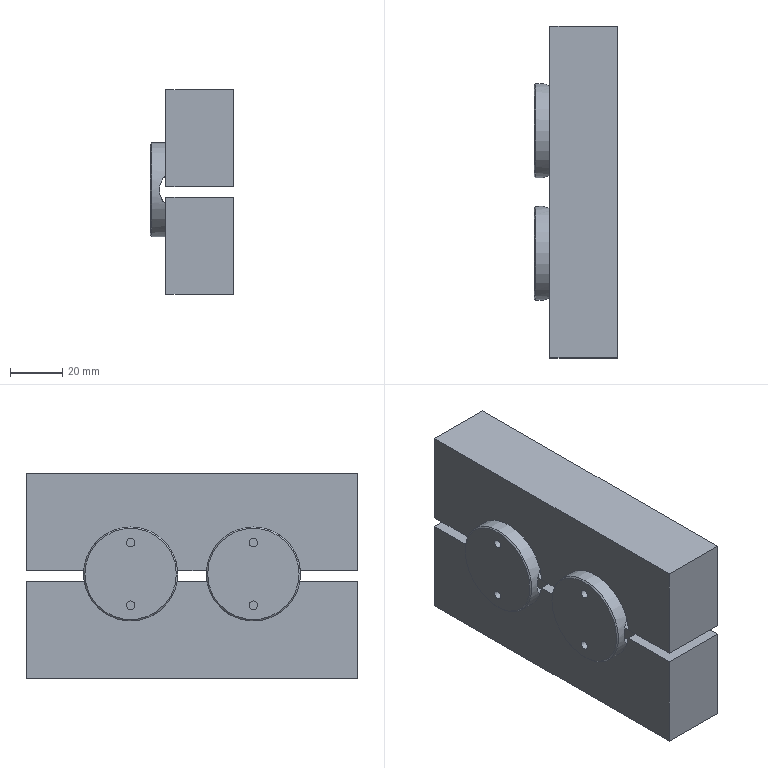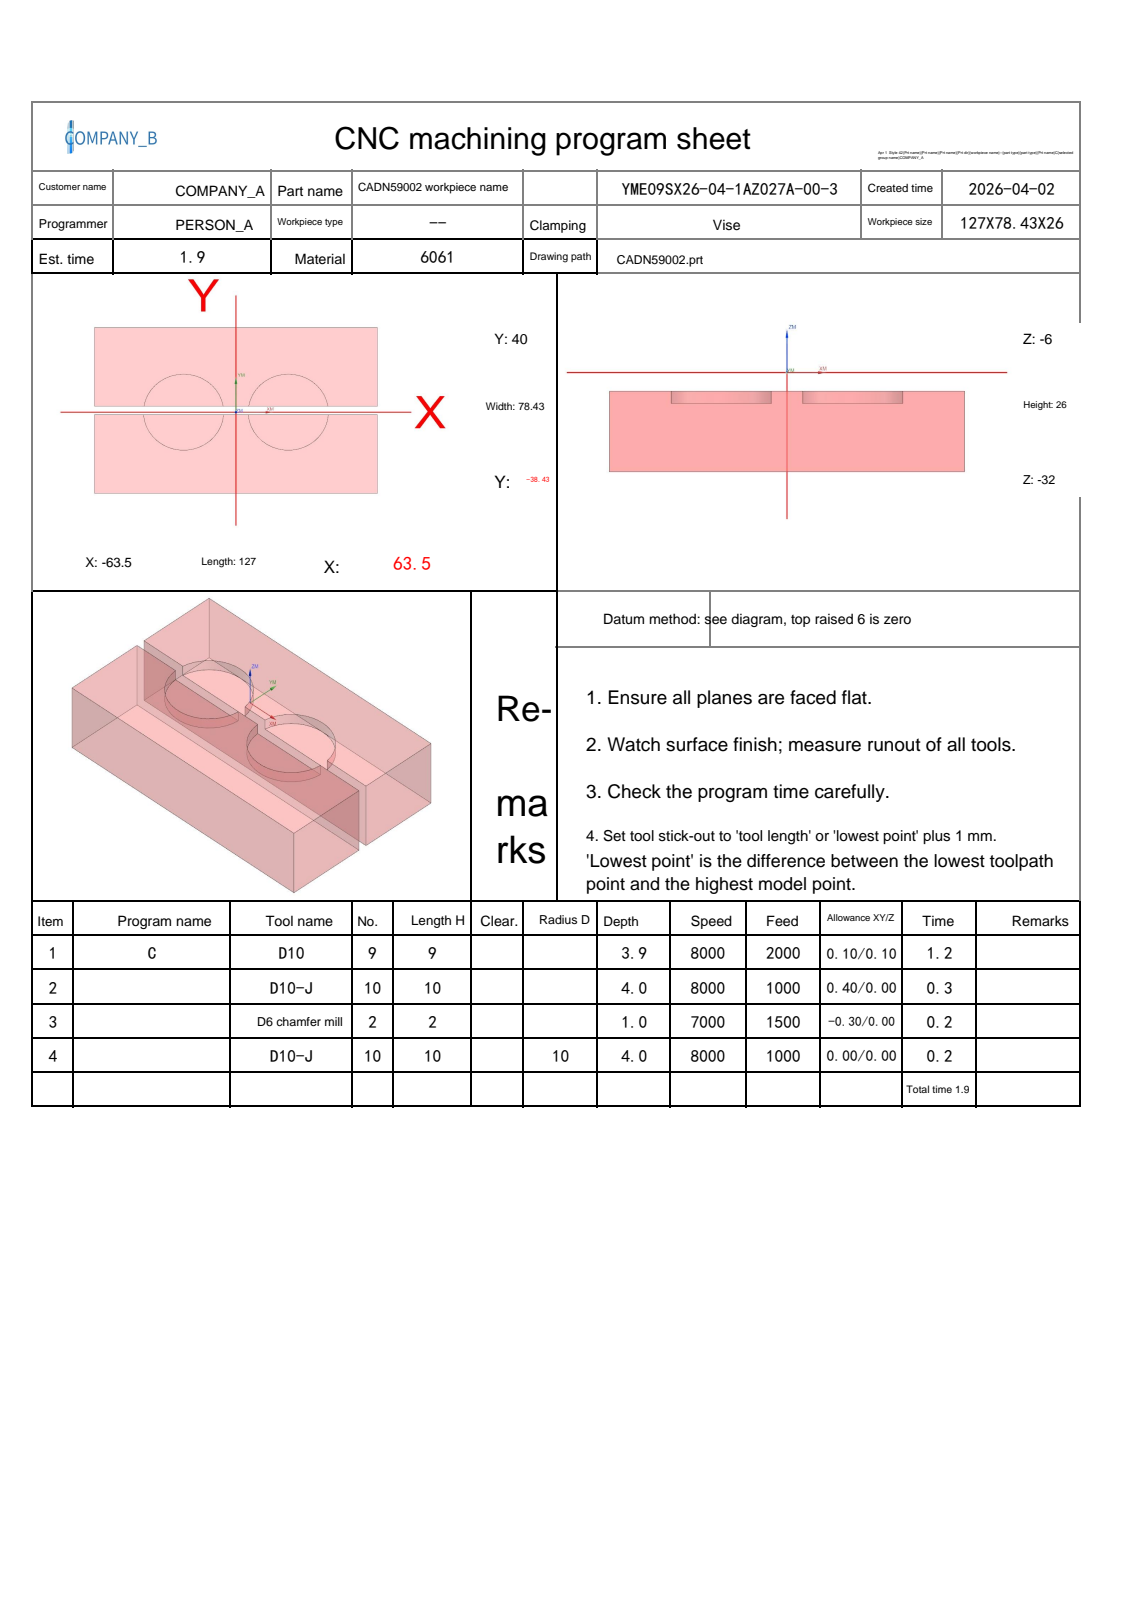NC program | NX | posted by the shop | part box 32 x 127 x 78.432 mm
Whole program:
%
O0001
(Machine time: 2.76 MIN)
(===Total Tool:3===)
(T9=D10     D=10.  R=0.   D-  H09 Z=-9.9  )
(T10=D10-J  D=10.  R=0.   D-  H10 Z=-10.  )
(T2=D6 chamfer mill   D=6.   R=0.   D-  H02 Z=-7.   )
G80 G90 G17 G49 G40
G91 G28 Z0
M01
N1 T09 M06
(D10  D=10. R=0. H=09 ce=0.10 di=0.10)
G00 G90 G54 X20.594 Y7.536 M03 S8000
G43 H09 Z4.1
M08
Z-4.5
G03 X20.594 Y7.536 Z-5.982 I2.906 J-3.436 F2000.
X23.5 Y-.4 Z-6.557 I2.906 J-3.436
G01 X23.527 Y-.399
G03 X23.9 Y0.0 I-.027 J.399
X23.5 Y.4 I-.4 J0.0
X23.1 Y0.0 I0.0 J-.4
G01 Y-.006
X23.11 Y-.041
X25.447 Y-4.037
G03 X26.224 Y-4.482 I.777 J.454
X26.768 Y-4.299 I0.0 J.9
X28.888 Y-.364 I-3.268 J4.299
G01 X28.921 Y.128
X28.923 Y.194
X28.911 Y.347
X28.835 Y.835
G03 X23.5 Y5.4 I-5.335 J-.835
X18.165 Y.834 I0.0 J-5.4
G01 X18.089 Y.347
X18.077 Y.194
X18.079 Y.128
X18.112 Y-.365
G03 X20.87 Y-4.716 I5.388 J.365
G02 X21.231 Y-5.059 I-.487 J-.873
G01 X25.608 Y-12.058
G03 X26.456 Y-12.527 I.848 J.531
X26.704 Y-12.496 I0.0 J1.
X36.371 Y-.871 I-3.204 J12.496
G01 X36.468 Y.569
X36.245 Y1.995
G03 X23.5 Y12.9 I-12.745 J-1.995
X10.755 Y1.995 I0.0 J-12.9
G01 X10.532 Y.569
X10.629 Y-.871
G03 X23.5 Y-12.9 I12.871 J.871
X28.376 Y-11.943 I0.0 J12.9
X28.835 Y-11.745 I-4.876 J11.943
G01 X27.594 Y-9.014
Z-5.057
G00 X20.594 Y7.536
G03 X20.594 Y7.536 Z-6.539 I2.906 J-3.436
X23.5 Y-.4 Z-7.114 I2.906 J-3.436
G01 X23.527 Y-.399
G03 X23.9 Y0.0 I-.027 J.399
X23.5 Y.4 I-.4 J0.0
X23.1 Y0.0 I0.0 J-.4
G01 Y-.006
X23.11 Y-.041
X25.447 Y-4.037
G03 X26.224 Y-4.482 I.777 J.454
X26.768 Y-4.299 I0.0 J.9
X28.888 Y-.364 I-3.268 J4.299
G01 X28.921 Y.128
X28.923 Y.194
X28.911 Y.347
X28.835 Y.835
G03 X23.5 Y5.4 I-5.335 J-.835
X18.165 Y.834 I0.0 J-5.4
G01 X18.089 Y.347
X18.077 Y.194
X18.079 Y.128
X18.112 Y-.365
G03 X20.87 Y-4.716 I5.388 J.365
G02 X21.231 Y-5.059 I-.487 J-.873
G01 X25.608 Y-12.058
G03 X26.456 Y-12.527 I.848 J.531
X26.704 Y-12.496 I0.0 J1.
X36.371 Y-.871 I-3.204 J12.496
G01 X36.468 Y.569
X36.245 Y1.995
G03 X23.5 Y12.9 I-12.745 J-1.995
X10.755 Y1.995 I0.0 J-12.9
G01 X10.532 Y.569
X10.629 Y-.871
G03 X23.5 Y-12.9 I12.871 J.871
X28.376 Y-11.943 I0.0 J12.9
X28.835 Y-11.745 I-4.876 J11.943
G01 X27.594 Y-9.014
Z-5.614
G00 X20.594 Y7.536
G03 X20.594 Y7.536 Z-7.096 I2.906 J-3.436
X23.5 Y-.4 Z-7.671 I2.906 J-3.436
G01 X23.527 Y-.399
G03 X23.9 Y0.0 I-.027 J.399
X23.5 Y.4 I-.4 J0.0
X23.1 Y0.0 I0.0 J-.4
G01 Y-.006
X23.11 Y-.041
X25.447 Y-4.037
G03 X26.224 Y-4.482 I.777 J.454
X26.768 Y-4.299 I0.0 J.9
X28.888 Y-.364 I-3.268 J4.299
G01 X28.921 Y.128
X28.923 Y.194
X28.911 Y.347
X28.835 Y.835
G03 X23.5 Y5.4 I-5.335 J-.835
X18.165 Y.834 I0.0 J-5.4
G01 X18.089 Y.347
X18.077 Y.194
X18.079 Y.128
X18.112 Y-.365
G03 X20.87 Y-4.716 I5.388 J.365
G02 X21.231 Y-5.059 I-.487 J-.873
G01 X25.608 Y-12.058
G03 X26.456 Y-12.527 I.848 J.531
X26.704 Y-12.496 I0.0 J1.
X36.371 Y-.871 I-3.204 J12.496
G01 X36.468 Y.569
X36.245 Y1.995
G03 X23.5 Y12.9 I-12.745 J-1.995
X10.755 Y1.995 I0.0 J-12.9
G01 X10.532 Y.569
X10.629 Y-.871
G03 X23.5 Y-12.9 I12.871 J.871
X28.376 Y-11.943 I0.0 J12.9
X28.835 Y-11.745 I-4.876 J11.943
G01 X27.594 Y-9.014
Z-6.171
G00 X20.594 Y7.536
G03 X20.594 Y7.536 Z-7.653 I2.906 J-3.436
X23.5 Y-.4 Z-8.229 I2.906 J-3.436
G01 X23.527 Y-.399
G03 X23.9 Y0.0 I-.027 J.399
X23.5 Y.4 I-.4 J0.0
X23.1 Y0.0 I0.0 J-.4
G01 Y-.006
X23.11 Y-.041
X25.447 Y-4.037
G03 X26.224 Y-4.482 I.777 J.454
X26.768 Y-4.299 I0.0 J.9
X28.888 Y-.364 I-3.268 J4.299
G01 X28.921 Y.128
X28.923 Y.194
X28.911 Y.347
X28.835 Y.835
G03 X23.5 Y5.4 I-5.335 J-.835
X18.165 Y.834 I0.0 J-5.4
G01 X18.089 Y.347
X18.077 Y.194
X18.079 Y.128
X18.112 Y-.365
G03 X20.87 Y-4.716 I5.388 J.365
G02 X21.231 Y-5.059 I-.487 J-.873
G01 X25.608 Y-12.058
G03 X26.456 Y-12.527 I.848 J.531
X26.704 Y-12.496 I0.0 J1.
X36.371 Y-.871 I-3.204 J12.496
G01 X36.468 Y.569
X36.245 Y1.995
G03 X23.5 Y12.9 I-12.745 J-1.995
X10.755 Y1.995 I0.0 J-12.9
G01 X10.532 Y.569
X10.629 Y-.871
G03 X23.5 Y-12.9 I12.871 J.871
X28.376 Y-11.943 I0.0 J12.9
X28.835 Y-11.745 I-4.876 J11.943
G01 X27.594 Y-9.014
Z-6.729
G00 X20.594 Y7.536
G03 X20.594 Y7.536 Z-8.21 I2.906 J-3.436
X23.5 Y-.4 Z-8.786 I2.906 J-3.436
G01 X23.527 Y-.399
G03 X23.9 Y0.0 I-.027 J.399
X23.5 Y.4 I-.4 J0.0
X23.1 Y0.0 I0.0 J-.4
G01 Y-.006
X23.11 Y-.041
X25.447 Y-4.037
G03 X26.224 Y-4.482 I.777 J.454
X26.768 Y-4.299 I0.0 J.9
X28.888 Y-.364 I-3.268 J4.299
G01 X28.921 Y.128
X28.923 Y.194
X28.911 Y.347
X28.835 Y.835
G03 X23.5 Y5.4 I-5.335 J-.835
X18.165 Y.834 I0.0 J-5.4
G01 X18.089 Y.347
X18.077 Y.194
X18.079 Y.128
X18.112 Y-.365
G03 X20.87 Y-4.716 I5.388 J.365
G02 X21.231 Y-5.059 I-.487 J-.873
G01 X25.608 Y-12.058
G03 X26.456 Y-12.527 I.848 J.531
X26.704 Y-12.496 I0.0 J1.
X36.371 Y-.871 I-3.204 J12.496
G01 X36.468 Y.569
X36.245 Y1.995
G03 X23.5 Y12.9 I-12.745 J-1.995
X10.755 Y1.995 I0.0 J-12.9
G01 X10.532 Y.569
X10.629 Y-.871
G03 X23.5 Y-12.9 I12.871 J.871
X28.376 Y-11.943 I0.0 J12.9
X28.835 Y-11.745 I-4.876 J11.943
G01 X27.594 Y-9.014
Z-7.286
G00 X20.594 Y7.536
G03 X20.594 Y7.536 Z-8.768 I2.906 J-3.436
X23.5 Y-.4 Z-9.343 I2.906 J-3.436
G01 X23.527 Y-.399
G03 X23.9 Y0.0 I-.027 J.399
X23.5 Y.4 I-.4 J0.0
X23.1 Y0.0 I0.0 J-.4
G01 Y-.006
X23.11 Y-.041
X25.447 Y-4.037
G03 X26.224 Y-4.482 I.777 J.454
X26.768 Y-4.299 I0.0 J.9
X28.888 Y-.364 I-3.268 J4.299
G01 X28.921 Y.128
X28.923 Y.194
X28.911 Y.347
X28.835 Y.835
G03 X23.5 Y5.4 I-5.335 J-.835
X18.165 Y.834 I0.0 J-5.4
G01 X18.089 Y.347
X18.077 Y.194
X18.079 Y.128
X18.112 Y-.365
G03 X20.87 Y-4.716 I5.388 J.365
G02 X21.231 Y-5.059 I-.487 J-.873
G01 X25.608 Y-12.058
G03 X26.456 Y-12.527 I.848 J.531
X26.704 Y-12.496 I0.0 J1.
X36.371 Y-.871 I-3.204 J12.496
G01 X36.468 Y.569
X36.245 Y1.995
G03 X23.5 Y12.9 I-12.745 J-1.995
X10.755 Y1.995 I0.0 J-12.9
G01 X10.532 Y.569
X10.629 Y-.871
G03 X23.5 Y-12.9 I12.871 J.871
X28.376 Y-11.943 I0.0 J12.9
X28.835 Y-11.745 I-4.876 J11.943
G01 X27.594 Y-9.014
Z-7.843
G00 X20.594 Y7.536
G03 X20.594 Y7.536 Z-9.325 I2.906 J-3.436
X23.5 Y-.4 Z-9.9 I2.906 J-3.436
G01 X23.527 Y-.399
G03 X23.9 Y0.0 I-.027 J.399
X23.5 Y.4 I-.4 J0.0
X23.1 Y0.0 I0.0 J-.4
G01 Y-.006
X23.11 Y-.041
X25.447 Y-4.037
G03 X26.224 Y-4.482 I.777 J.454
X26.768 Y-4.299 I0.0 J.9
X28.888 Y-.364 I-3.268 J4.299
G01 X28.921 Y.128
X28.923 Y.194
X28.911 Y.347
X28.835 Y.835
G03 X23.5 Y5.4 I-5.335 J-.835
X18.165 Y.834 I0.0 J-5.4
G01 X18.089 Y.347
X18.077 Y.194
X18.079 Y.128
X18.112 Y-.365
G03 X20.87 Y-4.716 I5.388 J.365
G02 X21.231 Y-5.059 I-.487 J-.873
G01 X25.608 Y-12.058
G03 X26.456 Y-12.527 I.848 J.531
X26.704 Y-12.496 I0.0 J1.
X36.371 Y-.871 I-3.204 J12.496
G01 X36.468 Y.569
X36.245 Y1.995
G03 X23.5 Y12.9 I-12.745 J-1.995
X10.755 Y1.995 I0.0 J-12.9
G01 X10.532 Y.569
X10.629 Y-.871
G03 X23.5 Y-12.9 I12.871 J.871
X28.376 Y-11.943 I0.0 J12.9
X28.835 Y-11.745 I-4.876 J11.943
G01 X27.594 Y-9.014
Z-8.4
G00 Z4.1
X-26.406 Y7.536
Z-4.5
G03 X-26.406 Y7.536 Z-5.982 I2.906 J-3.436
X-23.5 Y-.4 Z-6.557 I2.906 J-3.436
G01 X-23.473 Y-.399
G03 X-23.1 Y0.0 I-.027 J.399
X-23.5 Y.4 I-.4 J0.0
X-23.9 Y0.0 I0.0 J-.4
G01 Y-.006
X-23.89 Y-.041
X-21.553 Y-4.037
G03 X-20.776 Y-4.482 I.777 J.454
X-20.232 Y-4.299 I0.0 J.9
X-18.112 Y-.364 I-3.268 J4.299
G01 X-18.079 Y.128
X-18.077 Y.194
X-18.089 Y.347
X-18.165 Y.835
G03 X-23.5 Y5.4 I-5.335 J-.835
X-28.835 Y.834 I0.0 J-5.4
G01 X-28.911 Y.347
X-28.923 Y.194
X-28.921 Y.128
X-28.888 Y-.365
G03 X-26.13 Y-4.716 I5.388 J.365
G02 X-25.769 Y-5.059 I-.487 J-.873
G01 X-21.392 Y-12.058
G03 X-20.544 Y-12.527 I.848 J.531
X-20.296 Y-12.496 I0.0 J1.
X-10.629 Y-.871 I-3.204 J12.496
G01 X-10.532 Y.569
X-10.755 Y1.995
G03 X-23.5 Y12.9 I-12.745 J-1.995
X-36.245 Y1.995 I0.0 J-12.9
G01 X-36.468 Y.569
X-36.371 Y-.871
G03 X-23.5 Y-12.9 I12.871 J.871
X-18.624 Y-11.943 I0.0 J12.9
X-18.165 Y-11.745 I-4.876 J11.943
G01 X-19.406 Y-9.014
Z-5.057
G00 X-26.406 Y7.536
G03 X-26.406 Y7.536 Z-6.539 I2.906 J-3.436
X-23.5 Y-.4 Z-7.114 I2.906 J-3.436
G01 X-23.473 Y-.399
G03 X-23.1 Y0.0 I-.027 J.399
X-23.5 Y.4 I-.4 J0.0
X-23.9 Y0.0 I0.0 J-.4
G01 Y-.006
X-23.89 Y-.041
X-21.553 Y-4.037
G03 X-20.776 Y-4.482 I.777 J.454
X-20.232 Y-4.299 I0.0 J.9
X-18.112 Y-.364 I-3.268 J4.299
G01 X-18.079 Y.128
X-18.077 Y.194
X-18.089 Y.347
X-18.165 Y.835
G03 X-23.5 Y5.4 I-5.335 J-.835
X-28.835 Y.834 I0.0 J-5.4
G01 X-28.911 Y.347
X-28.923 Y.194
X-28.921 Y.128
X-28.888 Y-.365
G03 X-26.13 Y-4.716 I5.388 J.365
G02 X-25.769 Y-5.059 I-.487 J-.873
G01 X-21.392 Y-12.058
G03 X-20.544 Y-12.527 I.848 J.531
X-20.296 Y-12.496 I0.0 J1.
X-10.629 Y-.871 I-3.204 J12.496
G01 X-10.532 Y.569
X-10.755 Y1.995
G03 X-23.5 Y12.9 I-12.745 J-1.995
X-36.245 Y1.995 I0.0 J-12.9
G01 X-36.468 Y.569
X-36.371 Y-.871
G03 X-23.5 Y-12.9 I12.871 J.871
X-18.624 Y-11.943 I0.0 J12.9
X-18.165 Y-11.745 I-4.876 J11.943
G01 X-19.406 Y-9.014
Z-5.614
G00 X-26.406 Y7.536
G03 X-26.406 Y7.536 Z-7.096 I2.906 J-3.436
X-23.5 Y-.4 Z-7.671 I2.906 J-3.436
G01 X-23.473 Y-.399
G03 X-23.1 Y0.0 I-.027 J.399
X-23.5 Y.4 I-.4 J0.0
X-23.9 Y0.0 I0.0 J-.4
G01 Y-.006
X-23.89 Y-.041
X-21.553 Y-4.037
G03 X-20.776 Y-4.482 I.777 J.454
X-20.232 Y-4.299 I0.0 J.9
X-18.112 Y-.364 I-3.268 J4.299
G01 X-18.079 Y.128
X-18.077 Y.194
X-18.089 Y.347
X-18.165 Y.835
G03 X-23.5 Y5.4 I-5.335 J-.835
X-28.835 Y.834 I0.0 J-5.4
G01 X-28.911 Y.347
X-28.923 Y.194
X-28.921 Y.128
X-28.888 Y-.365
G03 X-26.13 Y-4.716 I5.388 J.365
G02 X-25.769 Y-5.059 I-.487 J-.873
G01 X-21.392 Y-12.058
G03 X-20.544 Y-12.527 I.848 J.531
X-20.296 Y-12.496 I0.0 J1.
X-10.629 Y-.871 I-3.204 J12.496
G01 X-10.532 Y.569
X-10.755 Y1.995
G03 X-23.5 Y12.9 I-12.745 J-1.995
X-36.245 Y1.995 I0.0 J-12.9
G01 X-36.468 Y.569
X-36.371 Y-.871
G03 X-23.5 Y-12.9 I12.871 J.871
X-18.624 Y-11.943 I0.0 J12.9
X-18.165 Y-11.745 I-4.876 J11.943
G01 X-19.406 Y-9.014
Z-6.171
G00 X-26.406 Y7.536
G03 X-26.406 Y7.536 Z-7.653 I2.906 J-3.436
X-23.5 Y-.4 Z-8.229 I2.906 J-3.436
G01 X-23.473 Y-.399
G03 X-23.1 Y0.0 I-.027 J.399
X-23.5 Y.4 I-.4 J0.0
X-23.9 Y0.0 I0.0 J-.4
G01 Y-.006
X-23.89 Y-.041
X-21.553 Y-4.037
G03 X-20.776 Y-4.482 I.777 J.454
X-20.232 Y-4.299 I0.0 J.9
X-18.112 Y-.364 I-3.268 J4.299
G01 X-18.079 Y.128
X-18.077 Y.194
X-18.089 Y.347
X-18.165 Y.835
G03 X-23.5 Y5.4 I-5.335 J-.835
X-28.835 Y.834 I0.0 J-5.4
G01 X-28.911 Y.347
X-28.923 Y.194
X-28.921 Y.128
X-28.888 Y-.365
G03 X-26.13 Y-4.716 I5.388 J.365
G02 X-25.769 Y-5.059 I-.487 J-.873
G01 X-21.392 Y-12.058
G03 X-20.544 Y-12.527 I.848 J.531
X-20.296 Y-12.496 I0.0 J1.
X-10.629 Y-.871 I-3.204 J12.496
G01 X-10.532 Y.569
X-10.755 Y1.995
G03 X-23.5 Y12.9 I-12.745 J-1.995
X-36.245 Y1.995 I0.0 J-12.9
G01 X-36.468 Y.569
X-36.371 Y-.871
G03 X-23.5 Y-12.9 I12.871 J.871
X-18.624 Y-11.943 I0.0 J12.9
X-18.165 Y-11.745 I-4.876 J11.943
G01 X-19.406 Y-9.014
Z-6.729
G00 X-26.406 Y7.536
G03 X-26.406 Y7.536 Z-8.21 I2.906 J-3.436
X-23.5 Y-.4 Z-8.786 I2.906 J-3.436
G01 X-23.473 Y-.399
G03 X-23.1 Y0.0 I-.027 J.399
X-23.5 Y.4 I-.4 J0.0
X-23.9 Y0.0 I0.0 J-.4
G01 Y-.006
X-23.89 Y-.041
X-21.553 Y-4.037
G03 X-20.776 Y-4.482 I.777 J.454
X-20.232 Y-4.299 I0.0 J.9
X-18.112 Y-.364 I-3.268 J4.299
G01 X-18.079 Y.128
X-18.077 Y.194
X-18.089 Y.347
X-18.165 Y.835
G03 X-23.5 Y5.4 I-5.335 J-.835
X-28.835 Y.834 I0.0 J-5.4
G01 X-28.911 Y.347
X-28.923 Y.194
X-28.921 Y.128
X-28.888 Y-.365
G03 X-26.13 Y-4.716 I5.388 J.365
G02 X-25.769 Y-5.059 I-.487 J-.873
G01 X-21.392 Y-12.058
G03 X-20.544 Y-12.527 I.848 J.531
X-20.296 Y-12.496 I0.0 J1.
X-10.629 Y-.871 I-3.204 J12.496
G01 X-10.532 Y.569
X-10.755 Y1.995
G03 X-23.5 Y12.9 I-12.745 J-1.995
X-36.245 Y1.995 I0.0 J-12.9
G01 X-36.468 Y.569
X-36.371 Y-.871
G03 X-23.5 Y-12.9 I12.871 J.871
X-18.624 Y-11.943 I0.0 J12.9
X-18.165 Y-11.745 I-4.876 J11.943
G01 X-19.406 Y-9.014
Z-7.286
G00 X-26.406 Y7.536
G03 X-26.406 Y7.536 Z-8.768 I2.906 J-3.436
X-23.5 Y-.4 Z-9.343 I2.906 J-3.436
G01 X-23.473 Y-.399
G03 X-23.1 Y0.0 I-.027 J.399
X-23.5 Y.4 I-.4 J0.0
X-23.9 Y0.0 I0.0 J-.4
G01 Y-.006
X-23.89 Y-.041
X-21.553 Y-4.037
G03 X-20.776 Y-4.482 I.777 J.454
X-20.232 Y-4.299 I0.0 J.9
X-18.112 Y-.364 I-3.268 J4.299
G01 X-18.079 Y.128
X-18.077 Y.194
X-18.089 Y.347
X-18.165 Y.835
G03 X-23.5 Y5.4 I-5.335 J-.835
X-28.835 Y.834 I0.0 J-5.4
G01 X-28.911 Y.347
X-28.923 Y.194
X-28.921 Y.128
X-28.888 Y-.365
G03 X-26.13 Y-4.716 I5.388 J.365
G02 X-25.769 Y-5.059 I-.487 J-.873
G01 X-21.392 Y-12.058
G03 X-20.544 Y-12.527 I.848 J.531
X-20.296 Y-12.496 I0.0 J1.
X-10.629 Y-.871 I-3.204 J12.496
G01 X-10.532 Y.569
X-10.755 Y1.995
G03 X-23.5 Y12.9 I-12.745 J-1.995
X-36.245 Y1.995 I0.0 J-12.9
G01 X-36.468 Y.569
X-36.371 Y-.871
G03 X-23.5 Y-12.9 I12.871 J.871
X-18.624 Y-11.943 I0.0 J12.9
X-18.165 Y-11.745 I-4.876 J11.943
G01 X-19.406 Y-9.014
Z-7.843
G00 X-26.406 Y7.536
G03 X-26.406 Y7.536 Z-9.325 I2.906 J-3.436
X-23.5 Y-.4 Z-9.9 I2.906 J-3.436
G01 X-23.473 Y-.399
G03 X-23.1 Y0.0 I-.027 J.399
X-23.5 Y.4 I-.4 J0.0
X-23.9 Y0.0 I0.0 J-.4
G01 Y-.006
X-23.89 Y-.041
X-21.553 Y-4.037
G03 X-20.776 Y-4.482 I.777 J.454
X-20.232 Y-4.299 I0.0 J.9
X-18.112 Y-.364 I-3.268 J4.299
G01 X-18.079 Y.128
X-18.077 Y.194
X-18.089 Y.347
X-18.165 Y.835
G03 X-23.5 Y5.4 I-5.335 J-.835
X-28.835 Y.834 I0.0 J-5.4
G01 X-28.911 Y.347
X-28.923 Y.194
X-28.921 Y.128
X-28.888 Y-.365
G03 X-26.13 Y-4.716 I5.388 J.365
G02 X-25.769 Y-5.059 I-.487 J-.873
G01 X-21.392 Y-12.058
G03 X-20.544 Y-12.527 I.848 J.531
X-20.296 Y-12.496 I0.0 J1.
X-10.629 Y-.871 I-3.204 J12.496
G01 X-10.532 Y.569
X-10.755 Y1.995
G03 X-23.5 Y12.9 I-12.745 J-1.995
X-36.245 Y1.995 I0.0 J-12.9
G01 X-36.468 Y.569
X-36.371 Y-.871
G03 X-23.5 Y-12.9 I12.871 J.871
X-18.624 Y-11.943 I0.0 J12.9
X-18.165 Y-11.745 I-4.876 J11.943
G01 X-19.406 Y-9.014
Z-8.4
G00 Z4.1
G91 G28 Z0.0
M05
M09
G91 G28 Z0.0
M01
N2 T10 M06
(D10-J  D=10. R=0. H=10 ce=0.40 di=0.00)
G00 G90 G54 X27.909 Y6.183 M03 S8000
G43 H10 Z4.4
M08
Z-8.
G01 X28.384 Y5.836 Z-8.158 F1000.
X29.117 Y5.134 Z-8.43
X29.751 Y4.341 Z-8.702
X30.273 Y3.47 Z-8.974
X30.674 Y2.538 Z-9.246
X30.948 Y1.561 Z-9.517
X31.14 Y.335 Z-9.85
X31.133 Y.226 Z-9.879
X31.102 Y-.224 Z-10.
X36.091 Y-.561
X36.071 Y-.851
G02 X23.5 Y-12.6 I-12.571 J.851
X10.929 Y-.851 I0.0 J12.6
G01 X10.841 Y.446
X10.839 Y.512
X10.85 Y.664
X11.052 Y1.949
G02 X23.5 Y12.6 I12.448 J-1.949
X35.948 Y1.949 I0.0 J-12.6
G01 X36.139 Y.733
X36.151 Y.579
G02 X35.52 Y-.35 I-1. J0.0
G01 X31.191 Y-2.069
G03 X30.623 Y-2.65 I.369 J-.929
G02 X23.5 Y-7.6 I-7.123 J2.65
X15.917 Y-.513 I0.0 J7.6
G01 X15.867 Y.226
X15.865 Y.291
X15.877 Y.443
X15.991 Y1.176
G02 X23.5 Y7.6 I7.509 J-1.176
X30.24 Y3.512 I0.0 J-7.6
X30.353 Y3.05 I-.887 J-.462
X29.884 Y2.203 I-1. J0.0
G01 X26.483 Y.068
G03 X26.039 Y-.562 I.532 J-.847
G02 X23.5 Y-2.6 I-2.539 J.562
X20.906 Y-.176 I0.0 J2.6
G01 X20.894 Y.006
X20.892 Y.071
X20.903 Y.223
X20.931 Y.402
G02 X23.5 Y2.6 I2.569 J-.402
X26.069 Y.402 I0.0 J-2.6
G01 X26.097 Y.223
X26.108 Y.096
X26.106 Y.006
X26.094 Y-.176
G02 X25.945 Y-.885 I-2.594 J.176
G03 X25.825 Y-1.566 I1.881 J-.681
X27.144 Y-3.447 I2. J0.0
G01 Z-8.5
G00 Z4.4
X-20.046 Y6.765
Z-8.
G01 X-19.436 Y6.434 Z-8.186
X-18.616 Y5.836 Z-8.458
X-17.883 Y5.134 Z-8.73
X-17.249 Y4.341 Z-9.002
X-16.727 Y3.47 Z-9.274
X-16.326 Y2.538 Z-9.546
X-16.052 Y1.561 Z-9.818
X-15.947 Y.889 Z-10.
X-11.007 Y1.662
X-10.851 Y.664
X-10.839 Y.512
X-10.841 Y.446
X-10.929 Y-.851
G02 X-23.5 Y-12.6 I-12.571 J.851
X-36.071 Y-.851 I0.0 J12.6
G01 X-36.159 Y.446
X-36.161 Y.512
X-36.149 Y.664
X-35.948 Y1.949
G02 X-23.5 Y12.6 I12.448 J-1.949
X-11.052 Y1.949 I0.0 J-12.6
G01 X-10.851 Y.664
X-10.839 Y.512
X-10.841 Y.446
X-10.929 Y-.851
G02 X-11.336 Y-3.284 I-12.571 J.851
X-12.256 Y-4.023 I-.965 J.261
G01 X-16.712 Y-4.223
G03 X-17.462 Y-4.615 I.045 J-.999
G02 X-23.5 Y-7.6 I-6.038 J4.615
X-31.083 Y-.513 I0.0 J7.6
G01 X-31.133 Y.226
X-31.135 Y.291
X-31.123 Y.444
X-31.009 Y1.176
G02 X-23.5 Y7.6 I7.509 J-1.176
X-16.039 Y1.449 I0.0 J-7.6
G01 X-16.021 Y1.259
G02 X-16.797 Y.284 I-1. J0.0
G01 X-20.466 Y-.558
G03 X-21.147 Y-1.106 I.224 J-.975
G02 X-23.5 Y-2.6 I-2.353 J1.106
X-26.094 Y-.176 I0.0 J2.6
G01 X-26.106 Y.005
X-26.108 Y.071
X-26.097 Y.223
X-26.069 Y.402
G02 X-23.5 Y2.6 I2.569 J-.402
X-20.931 Y.402 I0.0 J-2.6
G01 X-20.903 Y.223
X-20.892 Y.071
X-20.894 Y.005
X-20.906 Y-.176
G02 X-20.99 Y-.678 I-2.594 J.176
X-21.428 Y-1.57 I-2.51 J.678
G03 X-21.833 Y-2.778 I1.594 J-1.208
X-21.041 Y-4.372 I2. J0.0
G01 Z-8.5
G00 Z4.4
G91 G28 Z0.0
M05
M09
G91 G28 Z0.0
M01
N3 T02 M06
(D6 chamfer mill  D=6. R=0. H=02 ce=-0.30 di=0.00)
G00 G90 G54 X-7.557 Y-6.718 M03 S7000
G43 H02 Z44.
M08
Z-3.5
G01 X-7.256 Y-5.96 Z-3.797 F1500.
X-6.965 Y-5.097 Z-4.128
X-6.719 Y-4.22 Z-4.46
X-6.521 Y-3.331 Z-4.791
X-6.369 Y-2.433 Z-5.123
X-6.265 Y-1.529 Z-5.454
X-6.242 Y-1.207 Z-5.571
X-6.414 Y2.714 Z-7.
G03 X-23.5 Y17.3 I-17.086 J-2.714
X-40.8 Y0.0 I0.0 J-17.3
X-23.5 Y-17.3 I17.3 J0.0
X-6.242 Y-1.207 I0.0 J17.3
G01 X-6.414 Y2.714
G03 X-6.5 Y3.207 I-17.086 J-2.714
G01 Z-4.5
G00 Z44.
X39.445 Y-6.718
Z-3.5
G01 X39.763 Y-5.908 Z-3.817
X40.048 Y-5.054 Z-4.144
X40.289 Y-4.188 Z-4.472
X40.484 Y-3.309 Z-4.799
X40.633 Y-2.422 Z-5.127
X40.735 Y-1.529 Z-5.454
X40.758 Y-1.207 Z-5.571
X40.586 Y2.714 Z-7.
G03 X23.5 Y17.3 I-17.086 J-2.714
X6.2 Y0.0 I0.0 J-17.3
X23.5 Y-17.3 I17.3 J0.0
X40.758 Y-1.207 I0.0 J17.3
G01 X40.586 Y2.714
G03 X40.5 Y3.207 I-17.086 J-2.714
G01 Z-4.5
G00 Z44.
G91 G28 Z0.0
M05
M09
G91 G28 Z0.0
M01
N4 T10 M06
(D10-J  D=10. R=0. H=10 ce=0.00 di=0.00)
G00 G90 G54 X33.957 Y-2.713 M03 S8000
G43 H10 Z4.
M08
Z-9.
G01 Z-10. F1000.
G41 D10
X34.34 Y-2.738
X34.475 Y-2.743
G03 X36.47 Y-.878 I0.0 J2.
G01 X36.569 Y.573
X36.344 Y2.011
G03 X23.5 Y13. I-12.844 J-2.011
X10.656 Y2.011 I0.0 J-13.
G01 X10.431 Y.573
X10.53 Y-.878
G03 X23.5 Y-13. I12.97 J.878
X36.47 Y-.878 I0.0 J13.
G01 X36.497 Y-.479
X36.502 Y-.344
G03 X34.637 Y1.652 I-2. J0.0
G01 X34.373 Y1.669
G40 X34.173 Y1.683
Z-9.
G00 Z4.
X-33.68 Y3.618
Z-9.
G01 Z-10.
G41 D10
X-34.058 Y3.677
G03 X-34.368 Y3.701 I-.309 J-1.976
X-36.344 Y2.011 I0.0 J-2.
G01 X-36.569 Y.573
X-36.47 Y-.878
G03 X-23.5 Y-13. I12.97 J.878
X-10.53 Y-.878 I0.0 J13.
G01 X-10.431 Y.573
X-10.656 Y2.011
G03 X-23.5 Y13. I-12.844 J-2.011
X-36.344 Y2.011 I0.0 J-13.
G01 X-36.405 Y1.616
G03 X-36.429 Y1.306 I1.976 J-.309
X-34.739 Y-.67 I2. J0.0
G01 X-34.477 Y-.711
G40 X-34.279 Y-.742
Z-9.
G00 Z4.
M05
M09
G91 G28 Z0.0
G91 G28 Y0.0
M30
%